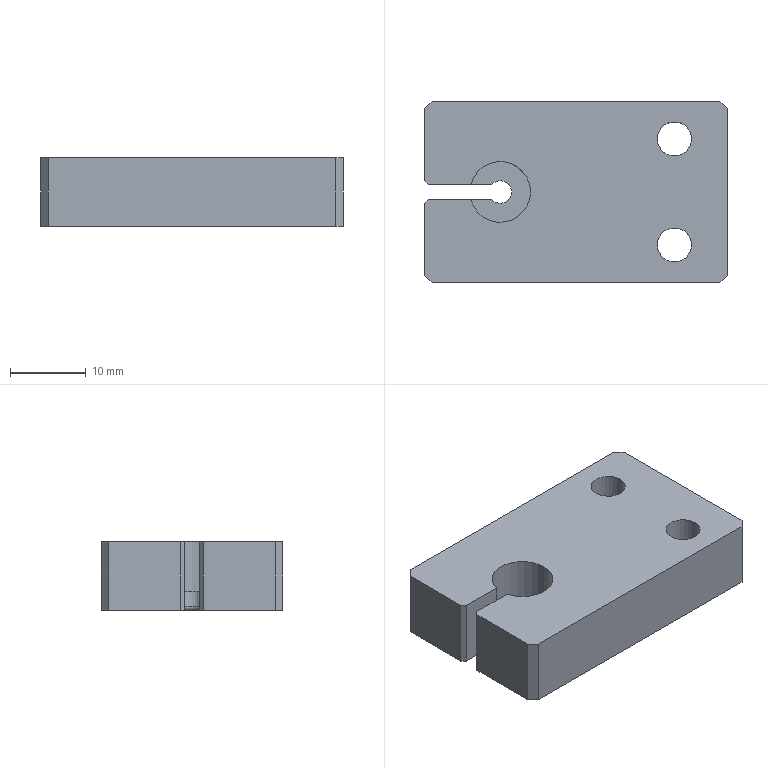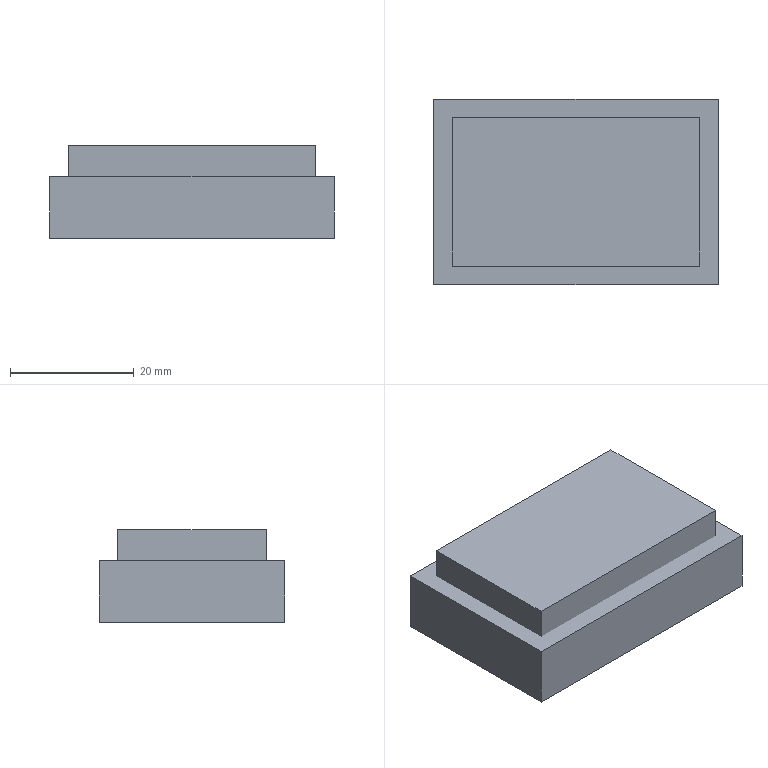CAM job | NX | 3-axis milling, drilling | part box 40 x 24 x 9 mm | stock box 46 x 30 x 15 mm
Tools:
number,name,description,diameter,corner_radius,flute_length,length,flutes
1,D63,Milling Tool-5 Parameters,63.0,0.0,50.0,75.0,2
9,D6A45,Milling Tool-5 Parameters,6.0,0.0,3.0,3.0,2
2,D10,Milling Tool-5 Parameters,10.0,0.0,50.0,75.0,2
14,4.5ZT,Drilling Tool,4.5,0.0,35.0,50.0,2
12,3.0ZT,Drilling Tool,3.0,0.0,35.0,50.0,2
4,D6,Milling Tool-5 Parameters,6.0,0.0,50.0,75.0,2
16,D1.5,Milling Tool-5 Parameters,1.5,0.0,50.0,75.0,2
Operations:
program,operation,operation_type,tool,method,geometry_group,spindle_rpm,surface_speed,feed_per_tooth,feed_cut,feed_plunge,cut_length_mm,path_length_mm,cut_time_min,machine_time_min
1-45-25-15虎钳,FLOOR_WALL,VolumeBased25DMillingOperation,D63,METHOD,A,6500.0,0.0,0.0,1250.0,100.0,121.0,175.0,0.0968,0.1022
1-45-25-15虎钳,DRILLING,Operation,D6A45,METHOD,A,4000.0,75.0,0.0312,250.0,0.0,12.0,128.546,0.048,0.0597
1-45-25-15虎钳,DRILLING_COPY_1,Operation,4.5ZT,METHOD,A,2000.0,20.0,0.05,200.0,0.0,21.704,120.726,0.1085,0.1184
1-45-25-15虎钳,DRILLING_COPY_1_COPY,Operation,3.0ZT,METHOD,A,2000.0,20.0,0.05,200.0,0.0,13.901,87.803,0.0695,0.0769
1-45-25-15虎钳,ADAPTIVE_MILLING,CavityMilling,D10,METHOD,A,7000.0,219.0,0.1429,2000.0,1000.0,662.611,734.611,0.3328,0.34
1-45-25-15虎钳,ZLEVEL_PROFILE_COPY_COPY_1_COPY,ZLevelMilling,D10,METHOD,A,6500.0,326.0,0.0769,1000.0,1000.0,166.12,241.12,0.1661,0.1736
1-45-25-15虎钳,HOLE_MILLING,CylinderMilling,D6,METHOD,A,5000.0,62.0,0.125,1250.0,100.0,114.413,179.913,0.0915,0.0981
1-45-25-15虎钳,ZLEVEL_PROFILE,ZLevelMilling,D1.5,METHOD,A,7000.0,32.0,0.0714,1000.0,100.0,1858.196,2025.678,1.858,1.875
1-45-25-15虎钳,ZLEVEL_PROFILE_COPY_1_COPY_COPY_COPY_COPY_COPY,ZLevelMilling,D6A45,METHOD,A,7000.0,131.0,0.0714,1000.0,1000.0,190.41,424.16,0.1904,0.2138
2-45-25-15虎钳,FLOOR_WALL_COPY,VolumeBased25DMillingOperation,D63,METHOD,B,6500.0,0.0,0.0,1250.0,100.0,690.0,1529.002,0.552,0.6359
2-45-25-15虎钳,HOLE_MILLING_COPY,CylinderMilling,D6,METHOD,B,5000.0,62.0,0.125,1250.0,100.0,158.833,298.834,0.1271,0.1411
2-45-25-15虎钳,ZLEVEL_PROFILE_COPY_1_COPY_COPY_COPY_COPY_COPY_COPY,ZLevelMilling,D6A45,METHOD,B,7000.0,131.0,0.0714,1000.0,1000.0,196.473,406.754,0.1965,0.2175
2-45-25-15虎钳,ZLEVEL_PROFILE_COPY,ZLevelMilling,D1.5,METHOD,B,7000.0,32.0,0.0714,1000.0,100.0,172.434,232.939,0.1724,0.1785